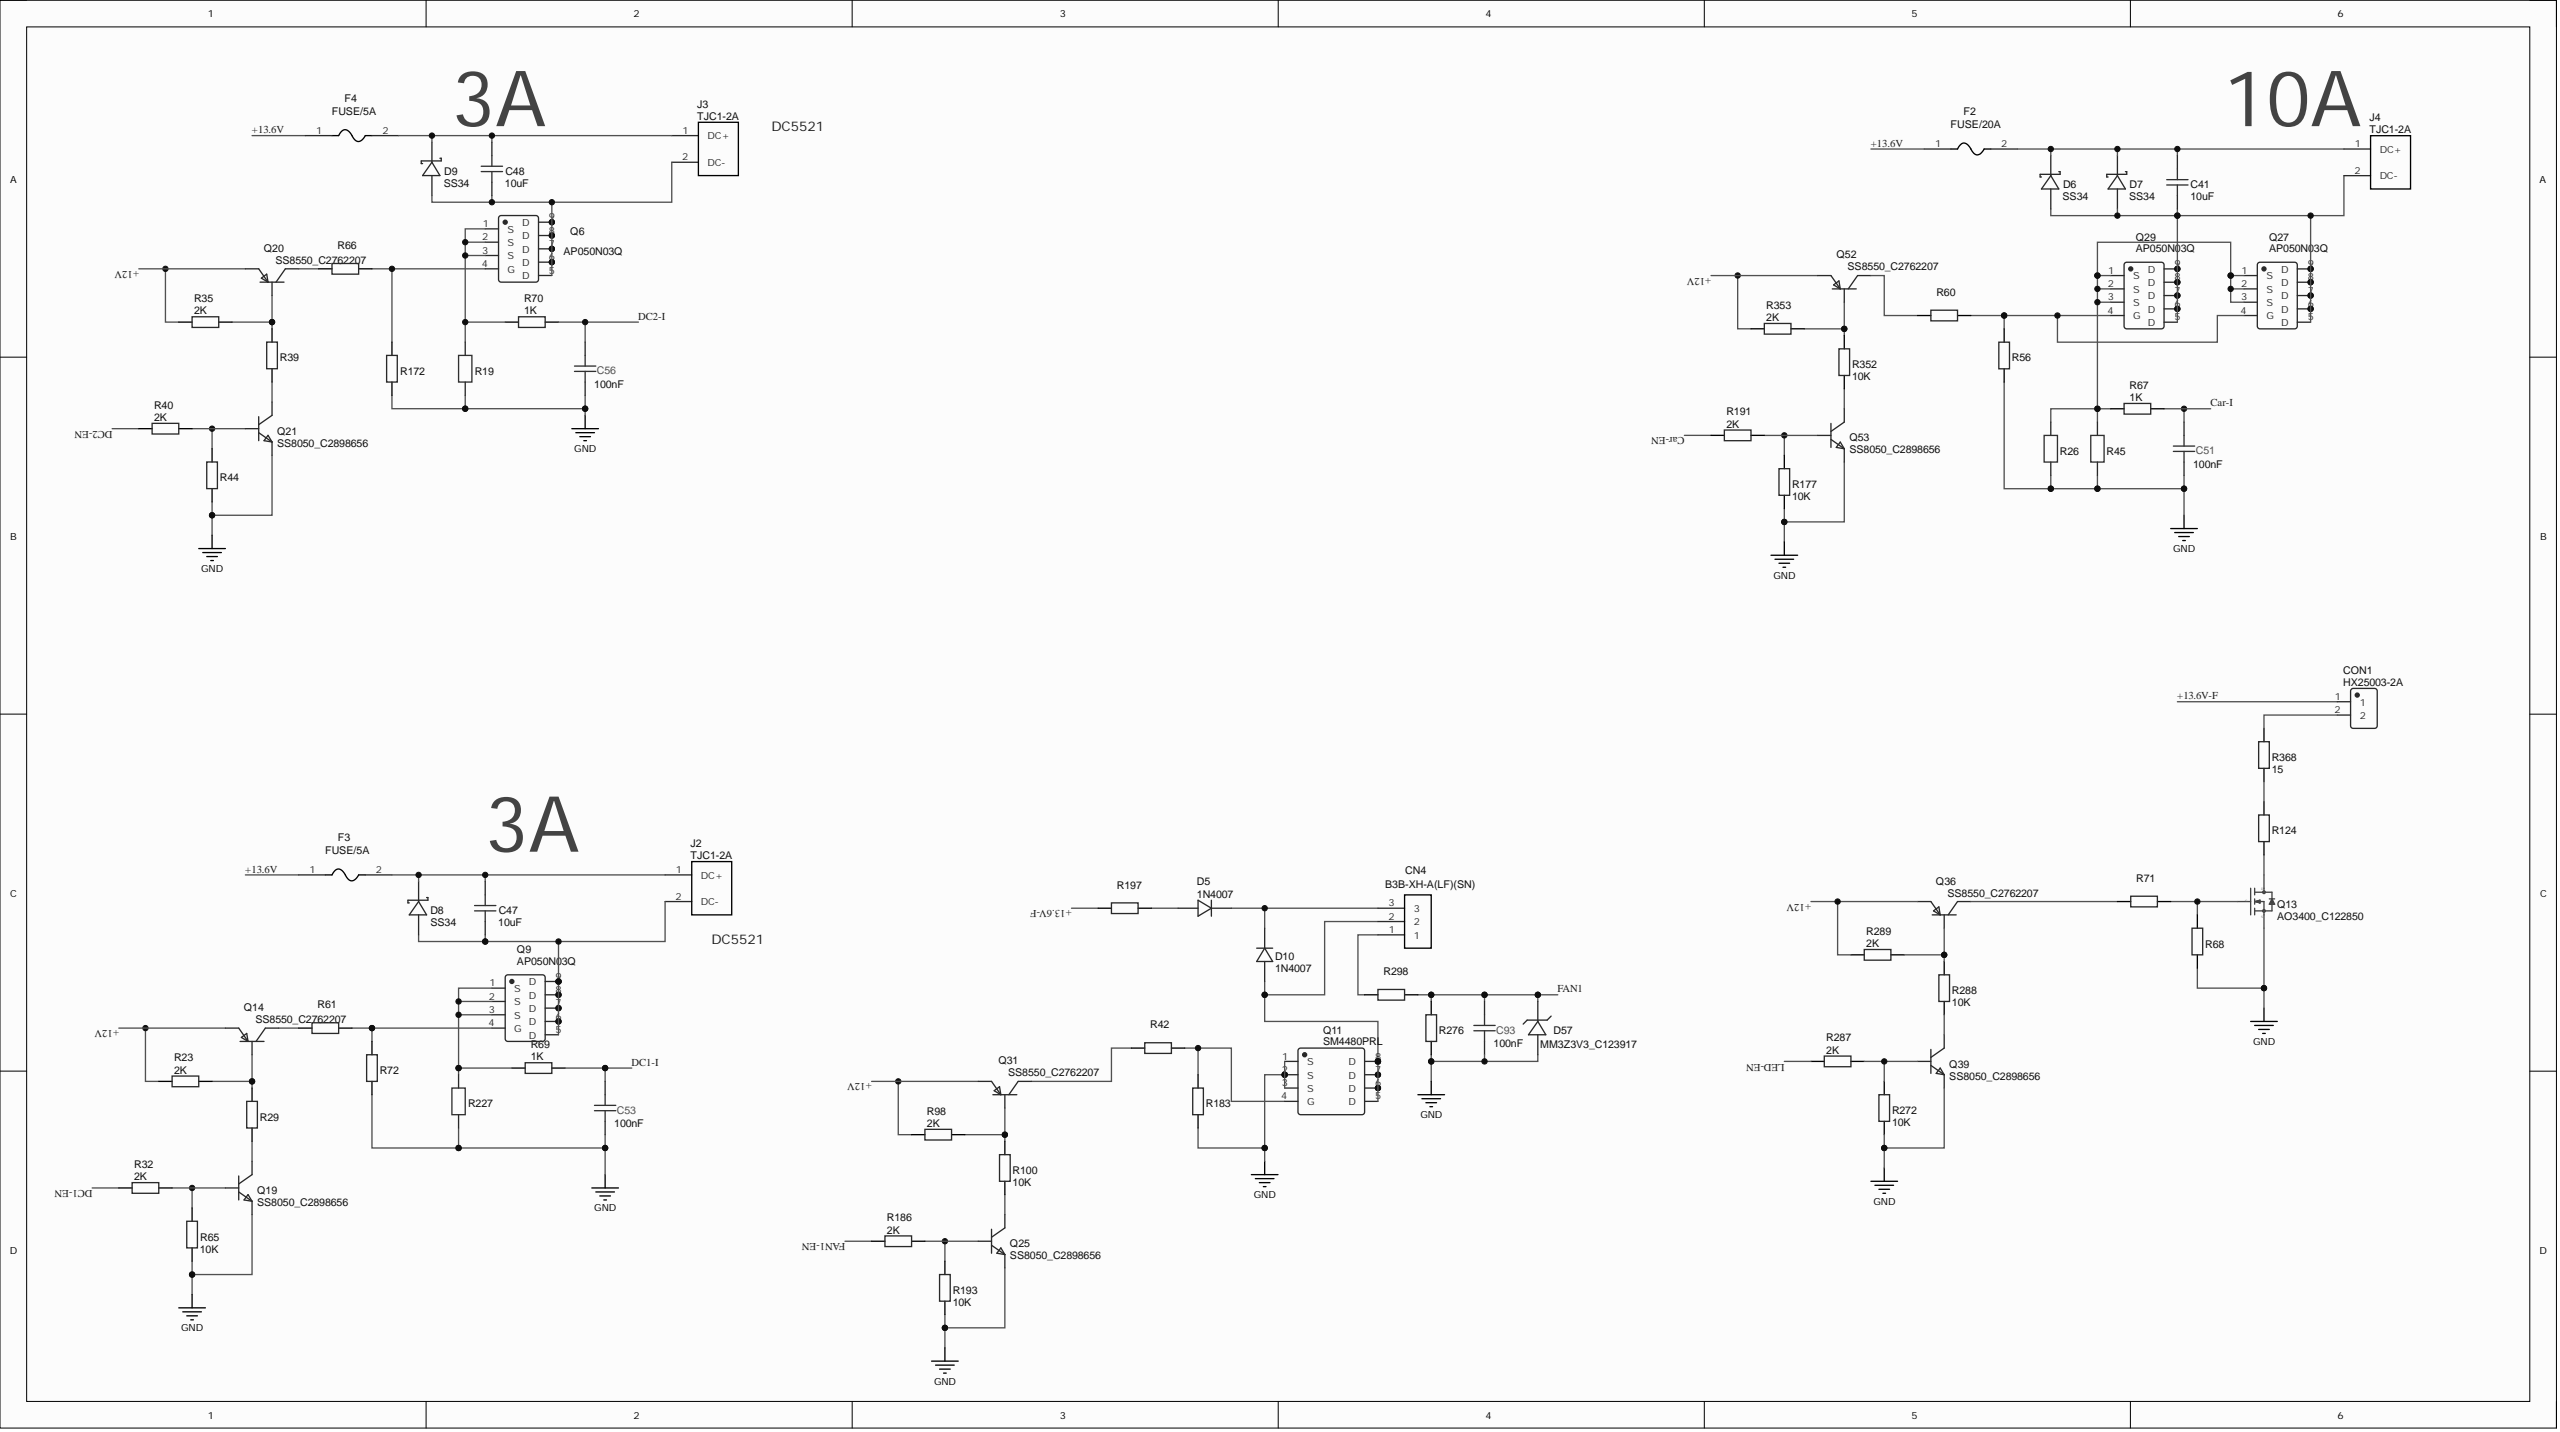Circuit board | Altium Designer | 694 parts | 423 nets | one sheet of the schematic
Parts on this sheet (reference | value | footprint):
C41 | 10uF | C0603
C47 | 10uF | C0603
C48 | 10uF | C0603
C51 | 100nF | C0603
C53 | 100nF | C0603
C56 | 100nF | C0603
C93 | 100nF | C0603
CN4 | B3B-XH-A(LF)(SN) | CONN-TH_3P-P2.50_B3B-XH-A-LF-SN
CON1 | HX25003-2A | CONN-TH_2P-P2.50_HX25003-2A
D5 | 1N4007 | DO-41_BD2.4-L4.7-P8.70-D0.9-RD
D6 | SS34 | SMC_L7.1-W6.2-LS8.1-R-RD
D7 | SS34 | SMC_L7.1-W6.2-LS8.1-R-RD
D8 | SS34 | SMC_L7.1-W6.2-LS8.1-R-RD
D9 | SS34 | SMC_L7.1-W6.2-LS8.1-R-RD
D10 | 1N4007 | DO-41_BD2.4-L4.7-P8.70-D0.9-RD
D57 | MM3Z3V3_C123917 | SOD-323_L1.8-W1.3-LS2.5-RD
F2 | FUSE/20A | FUSE-SMD_L6.1-W2.5
F3 | FUSE/5A | FUSE-SMD_L6.1-W2.5
F4 | FUSE/5A | FUSE-SMD_L6.1-W2.5
J2 | TJC1-2A | DC5521
J3 | TJC1-2A | DC5521
J4 | TJC1-2A | CONN-TH_XT60UPB-F-W
Q6 | AP050N03Q | PDFN-8_L3.1-W3.1-P0.65-LS3.4-BL
Q9 | AP050N03Q | PDFN-8_L3.1-W3.1-P0.65-LS3.4-BL
Q11 | SM4480PRL | SOP-8_L4.9-W3.9-P1.27-LS6.0-BL
Q13 | AO3400_C122850 | SC-59-3_L2.9-W1.5-P0.95-LS2.5-BR
Q14 | SS8550_C2762207 | SOT-23-3_L2.9-W1.3-P1.90-LS2.4-BR
Q19 | SS8050_C2898656 | SOT-23-3_L2.9-W1.3-P1.90-LS2.4-BR
Q20 | SS8550_C2762207 | SOT-23-3_L2.9-W1.3-P1.90-LS2.4-BR
Q21 | SS8050_C2898656 | SOT-23-3_L2.9-W1.3-P1.90-LS2.4-BR
Q25 | SS8050_C2898656 | SOT-23-3_L2.9-W1.3-P1.90-LS2.4-BR
Q27 | AP050N03Q | PDFN-8_L3.1-W3.1-P0.65-LS3.4-BL
Q29 | AP050N03Q | PDFN-8_L3.1-W3.1-P0.65-LS3.4-BL
Q31 | SS8550_C2762207 | SOT-23-3_L2.9-W1.3-P1.90-LS2.4-BR
Q36 | SS8550_C2762207 | SOT-23-3_L2.9-W1.3-P1.90-LS2.4-BR
Q39 | SS8050_C2898656 | SOT-23-3_L2.9-W1.3-P1.90-LS2.4-BR
Q52 | SS8550_C2762207 | SOT-23-3_L2.9-W1.3-P1.90-LS2.4-BR
Q53 | SS8050_C2898656 | SOT-23-3_L2.9-W1.3-P1.90-LS2.4-BR
R19 | RES-SMD_L6.4-W3.2-R2512
R23 | 2K | R0603
R26 | R2512
R29 | R0603
R32 | 2K | R0603
R35 | 2K | R0603
R39 | R0603
R40 | 2K | R0603
R42 | R0603
R44 | R0603
R45 | R2512
R56 | R0603
R60 | R0603
R61 | R0603
R65 | 10K | R0603
R66 | R0603
R67 | 1K | R0603
R68 | R0603
R69 | 1K | R0603
R70 | 1K | R0603
R71 | R0603
R72 | R0603
R98 | 2K | R0603
R100 | 10K | R0603
R124 | R0603
R172 | R0603
R177 | 10K | R0603
R183 | R0603
R186 | 2K | R0603
R191 | 2K | R0603
R193 | 10K | R0603
R197 | R0603
R227 | RES-SMD_L6.4-W3.2-R2512
R272 | 10K | R0603
R276 | R0603
R287 | 2K | R0603
R288 | 10K | R0603
R289 | 2K | R0603
R298 | R0603
R352 | 10K | R0603
R353 | 2K | R0603
R368 | 15 | r2512
Nets of these parts (net: part-pin ...):
NetR124_2: R124-2 R368-1
NetQ53_3: Q53-3 R352-1
NetQ53_1: Q53-1 R177-1 R191-2
NetQ52_3: Q52-3 R60-1
NetQ52_1: Q52-1 R352-2 R353-2
NetQ39_3: Q39-3 R288-1
NetQ39_1: Q39-1 R272-1 R287-2
NetQ36_3: Q36-3 R71-1
NetQ36_1: Q36-1 R288-2 R289-2
NetQ31_3: Q31-3 R42-1
NetQ31_1: Q31-1 R98-2 R100-2
NetQ27_4: Q27-4 Q29-4 R56-2 R60-2
NetQ27_1: Q27-1 Q27-2 Q27-3 Q29-1 Q29-2 Q29-3 R26-2 R45-2 R67-1
NetQ25_3: Q25-3 R100-1
NetQ25_1: Q25-1 R186-2 R193-1
NetQ21_3: Q21-3 R39-2
NetQ21_1: Q21-1 R40-2 R44-1
NetQ20_3: Q20-3 R66-1
NetQ20_1: Q20-1 R35-2 R39-1
NetQ19_3: Q19-3 R29-2
NetQ19_1: Q19-1 R32-2 R65-1
NetQ14_3: Q14-3 R61-1
NetQ14_1: Q14-1 R23-2 R29-1
NetQ13_3: Q13-3 R124-1
NetQ13_1: Q13-1 R68-2 R71-2
NetQ11_4: Q11-4 R42-2 R183-2
NetQ9_4: Q9-4 R61-2 R72-1
NetQ9_1: Q9-1 Q9-2 Q9-3 R69-1 R227-2
NetQ6_4: Q6-4 R66-2 R172-2
NetQ6_1: Q6-1 Q6-2 Q6-3 R19-2 R70-1
NetD5_2: D5-2 R197-2
NetCON1_2: CON1-2 R368-2
NetCN4_3: CN4-3 D5-1 D10-1
NetCN4_2: CN4-2 D10-2 Q11-5 Q11-6 Q11-7 Q11-8
NetCN4_1: CN4-1 R298-1
NetC48_2: C48-2 D9-2 F4-2 J3-1
NetC48_1: C48-1 D9-1 J3-2 Q6-5 Q6-6 Q6-7 Q6-8 Q6-9
NetC47_2: C47-2 D8-2 F3-2 J2-1
NetC47_1: C47-1 D8-1 J2-2 Q9-5 Q9-6 Q9-7 Q9-8 Q9-9
NetC41_2: C41-2 D6-2 D7-2 F2-2 J4-1
NetC41_1: C41-1 D6-1 D7-1 J4-2 Q27-5 Q27-6 Q27-7 Q27-8 Q27-9 Q29-5 Q29-6 Q29-7 Q29-8 Q29-9
LED-EN: R287-1
GND: C51-1 C53-1 C56-1 C93-1 D57-2 Q11-1 Q11-2 Q11-3 Q13-2 Q19-2 Q21-2 Q25-2 Q39-2 Q53-2 R19-1 R26-1 R44-2 R45-1 R56-1 R65-2 R68-1 R72-2 R172-1 R177-2 R183-1 R193-2 R227-1 R272-2 R276-1
FAN1-EN: R186-1
FAN1: C93-2 D57-1 R276-2 R298-2
DC2-I: C56-2 R70-2
DC2-EN: R40-1
DC1-I: C53-2 R69-2
DC1-EN: R32-1
Car-I: C51-2 R67-2
Car-EN: R191-1
+13.6V-F: CON1-1 R197-1
+13.6V: F2-1 F3-1 F4-1
+12V: Q14-2 Q20-2 Q31-2 Q36-2 Q52-2 R23-1 R35-1 R98-1 R289-1 R353-1